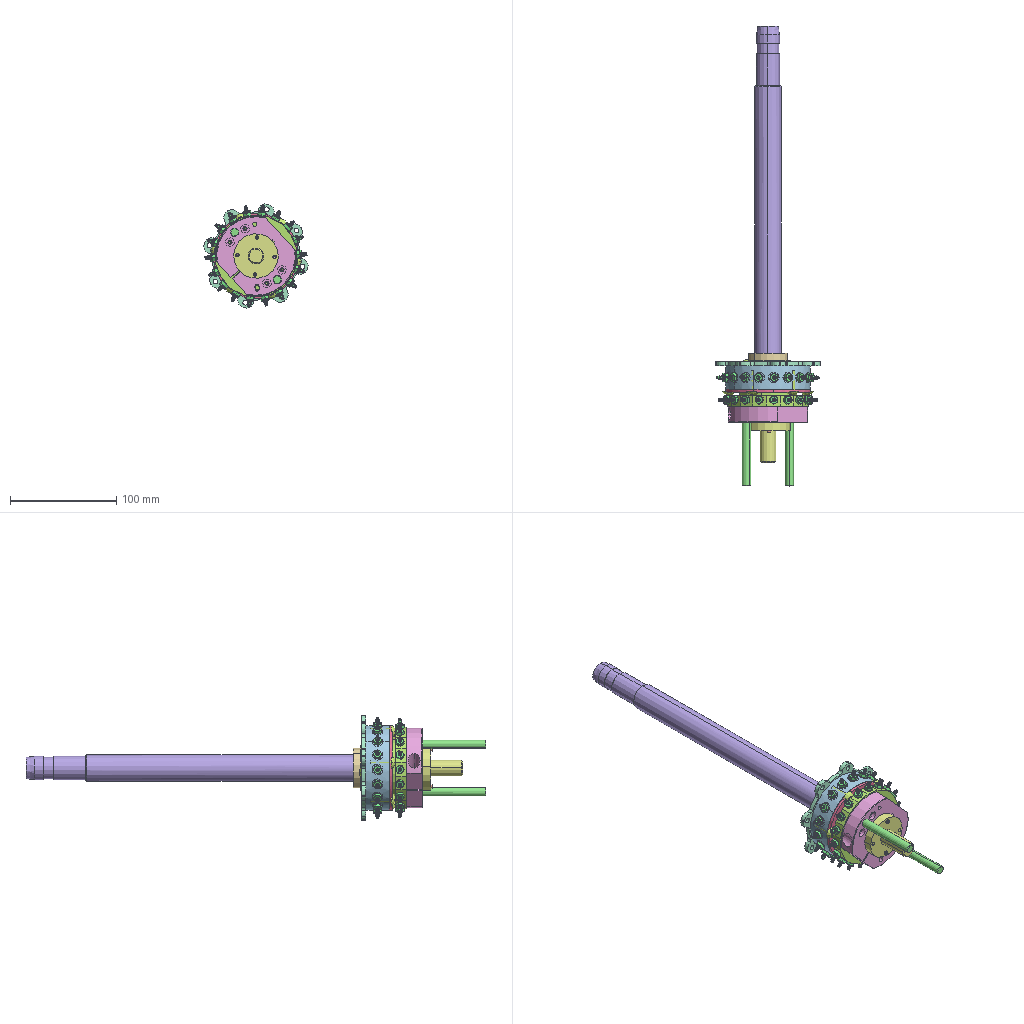Assembly | SolidWorks | 25 different items | 116 placed | box 98 x 433 x 98 mm
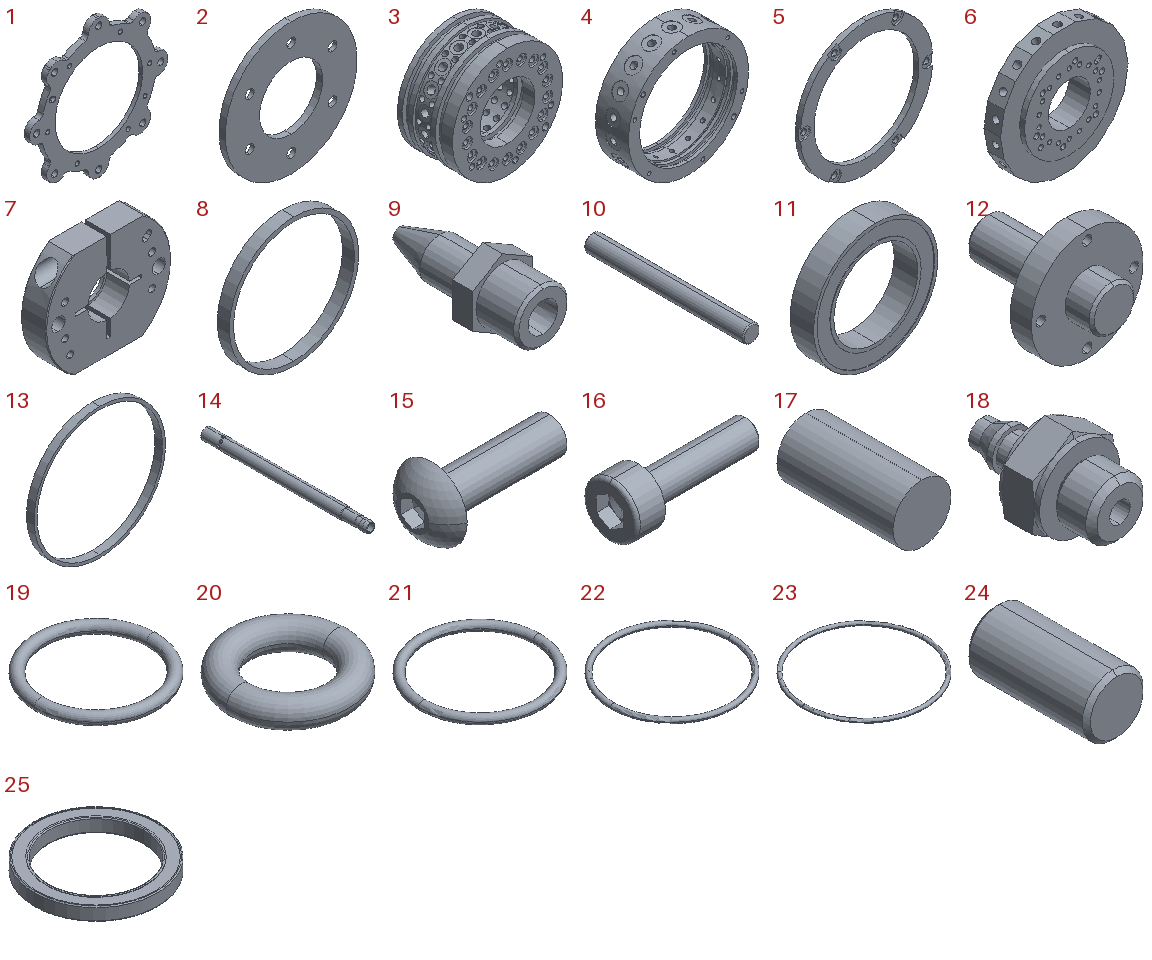Parts list (item | quantity | size | volume | features):
1 | x1 | 100 x 4 x 100 mm | 10292 mm3 | features ICE 11, CirPattern 3, Fillet 2, Extrusion 1
2 | x1 | 52.5 x 2.5 x 52.5 mm | 3777 mm3 | features ICE 4, CirPattern 2, Chamfer 1, Extrusion 1
3 | x1 | 50 x 25 x 50 mm | 28729 mm3 | features ICE 10, CirPattern 7, RevCut 4, 3DProfileFeature 3, HoleWzd 3, Extrusion 1
4 | x1 | 80 x 22 x 80 mm | 34396 mm3 | features ICE 6, CirPattern 5, 3DProfileFeature 3, HoleWzd 3, RevCut 2, Cut 1, Extrusion 1, Revolution 1
5 | x1 | 80 x 3 x 80 mm | 5249 mm3 | features CirPattern 3, ICE 2, Cut 1, Extrusion 1
6 | x1 | 77.172 x 13 x 76 mm | 40512 mm3 | features ICE 12, CirPattern 5, HoleWzd 2, 3DProfileFeature 1, Chamfer 1, Cut 1, Extrusion 1
7 | x1 | 75 x 15 x 62 mm | 46080 mm3 | features ICE 12, 3DProfileFeature 2, HoleWzd 2, Chamfer 1, CirPattern 1, Extrusion 1
8 | x1 | 27 x 2.5 x 27 mm | 184.49 mm3 | features Extrusion 1
9 | x18 | 4.5 x 10.7 x 5.196 mm | 80.12 mm3 | features ICE 4, Chamfer 2, Extrusion 1, RevCut 1
10 | x2 | 8 x 75 x 8 mm | 3753 mm3 | features Chamfer 1, Extrusion 1, ICE 1
11 | x1 | 37 x 7 x 37 mm | 3935 mm3 | features ICE 2, Extrusion 1
12 | x1 | 42 x 48 x 42 mm | 18246 mm3 | features ICE 10, Chamfer 2, CirPattern 2, Extrusion 1
13 | x1 | 52.5 x 3 x 52.5 mm | 556.557 mm3 | features Extrusion 1
14 | x1 | 25 x 371 x 25 mm | 90004 mm3 | features Chamfer 3, ICE 3, CirPattern 2, Extrusion 1, RefAxis 1, RevCut 1
15 | x14 | 23.3 x 12 x 12 mm | 775.96 mm3 | features Cut 2, RevCut 2, Boss 1, Extrusion 1, Fillet 1, LPattern 1
16 | x2 | 7.6 x 3 x 3 mm | 21.652 mm3 | features Fillet 2, RevCut 2, Boss 1, Chamfer 1, Cut 1, Extrusion 1, LPattern 1
17 | x2 | 4 x 8 x 4 mm | 100.531 mm3 | features Extrusion 1
18 | x36 | 7 x 12 x 8.083 mm | 212.301 mm3 | features BaseBody 1
19 | x1 | 22 x 22 x 2 mm | 197.392 mm3 | features RefAxis 1, Revolution 1
20 | x18 | 4.6 x 4.6 x 1 mm | 8.883 mm3 | features RefAxis 1, Revolution 1
21 | x2 | 29 x 29 x 2 mm | 266.479 mm3 | features RefAxis 1, Revolution 1
22 | x2 | 50 x 50 x 2 mm | 473.741 mm3 | features RefAxis 1, Revolution 1
23 | x2 | 69 x 69 x 2 mm | 661.263 mm3 | features RefAxis 1, Revolution 1
24 | x3 | 3 x 6 x 3 mm | 42.051 mm3 | features Chamfer 1, Extrusion 1
25 | x2 | 65 x 65 x 7 mm | 9064 mm3 | features Extrusion 1, Fillet 1, ICE 1, MirrorPattern 1
Mates (type | each side: item.copy, entity, surface, feature):
DistanceDim | 3.1 face plane Boss-Extrude1 | 2.1 face plane Boss-Extrude1
Concentric | 2.1 face cylinder Boss-Extrude1 | 3.1 face cylinder Boss-Extrude1
Concentric | 2.1 face cylinder CirPattern1 | 3.1 face cylinder M3 Tapped Hole1
Coincident | 2.1 face plane Boss-Extrude1 | 25.1 face plane Boss-Extrude1
Coincident | 4.1 face plane Boss-Extrude1 | 5.1 face plane Boss-Extrude1
Concentric | 4.1 face cylinder Boss-Extrude1 | 5.1 face cylinder Boss-Extrude1
Concentric | 4.1 face cylinder Boss-Extrude1 | 25.2 face cylinder Boss-Extrude1
Coincident | 4.1 face plane Revolve1 | 25.2 face plane Boss-Extrude1
Coincident | 4.1 face plane Revolve1 | 25.1 face plane Boss-Extrude1
Concentric | 4.1 face cylinder Boss-Extrude1 | 25.1 face cylinder Boss-Extrude1
Concentric | 3.1 face cylinder Boss-Extrude1 | 25.2 face cylinder Boss-Extrude1
Concentric | 7.1 face cylinder Cut-Extrude8 | 10.1 face cylinder Boss-Extrude1
Coincident | 10.1 face plane Boss-Extrude1 | 10.2 face plane Boss-Extrude1
DistanceDim | 10.2 face plane Boss-Extrude1 | 6.1 face plane Boss-Extrude3
Coincident | 4.1 face plane CirPattern2 | 18.1 face plane Input 1
Concentric | 4.1 face cylinder CirPattern3 | 18.1 face cylinder Input 1
Coincident | 6.1 face plane Boss-Extrude3 | 18.2 face plane Input 1
Concentric | 6.1 face cylinder CirPattern14 | 18.2 face cylinder Input 1
Coincident | 12.1 face plane Boss-Extrude1 | 16.1 face plane BaseHead
Coincident | 12.1 face plane Boss-Extrude1 | 16.2 face plane BaseHead
Coincident | 3.1 face plane CirPattern6 | 9.1 face plane Boss-Extrude2
DistanceDim | 22.1 plane | 3.1 face plane Cut-Revolve2
DistanceDim | 22.2 plane | 3.1 face plane Cut-Revolve2
DistanceDim | 23.1 plane | 4.1 face plane Cut-Revolve3
DistanceDim | 23.2 plane | 4.1 face plane Cut-Revolve3
Concentric | 3.1 face cylinder CirPattern11 | 9.1 face cylinder Boss-Extrude3
DistanceDim | 3.1 face plane CirPattern13 | 20.1 plane
Concentric | 3.1 edge | 20.1 axis
Coincident | 3.1 face plane Cut-Extrude12 | 24.1 face plane Boss-Extrude1
Concentric | 3.1 face cylinder Cut-Extrude12 | 24.1 face cylinder Boss-Extrude1
Coincident | 3.1 face plane Cut-Extrude12 | 24.2 face plane Boss-Extrude1
Concentric | 3.1 face cylinder Cut-Extrude12 | 24.2 face cylinder Boss-Extrude1
Parallel | 4.1 face plane CirPattern2 | 6.1 face plane Boss-Extrude3
Coincident | 4.1 face plane Cut-Extrude7 | 24.3 face plane Boss-Extrude1
Concentric | 4.1 face cylinder Cut-Extrude7 | 24.3 face cylinder Boss-Extrude1
Coincident | 1.1 face plane Boss-Extrude1 | 4.1 face plane Boss-Extrude1
Concentric | 1.1 face cylinder Cut-Extrude1 | 4.1 face cylinder Boss-Extrude1
Coincident | 6.1 face plane Cut-Extrude14 | 17.1 face plane Boss-Extrude1
Concentric | 6.1 face cylinder Cut-Extrude14 | 17.1 face cylinder Boss-Extrude1
Coincident | 6.1 face plane Cut-Extrude14 | 17.2 face plane Boss-Extrude1
Concentric | 6.1 face cylinder Cut-Extrude14 | 17.2 face cylinder Boss-Extrude1
Concentric | 3.1 edge | 21.1 axis
DistanceDim | 21.1 plane | 3.1 face plane Cut-Revolve3
Concentric | 3.1 edge | 21.2 axis
DistanceDim | 21.2 plane | 3.1 face plane Cut-Revolve3
Concentric | 3.1 face cylinder Boss-Extrude1 | 13.1 face cylinder Boss-Extrude1
Concentric | 2.1 face cylinder Cut-Extrude2 | 15.1 face cylinder BaseBody
Coincident | 2.1 face plane Cut-Extrude3 | 15.1 face plane BaseHead
Concentric | 2.1 face cylinder CirPattern1 | 15.2 face cylinder BaseBody
Coincident | 2.1 face plane CirPattern2 | 15.2 face plane BaseHead
Concentric | 2.1 face cylinder CirPattern1 | 15.3 face cylinder BaseBody
Coincident | 2.1 face plane CirPattern2 | 15.3 face plane BaseHead
Concentric | 2.1 face cylinder CirPattern1 | 15.4 face cylinder BaseBody
Coincident | 2.1 face plane CirPattern2 | 15.4 face plane BaseHead
Concentric | 2.1 face cylinder CirPattern1 | 15.5 face cylinder BaseBody
Coincident | 2.1 face plane CirPattern2 | 15.5 face plane BaseHead
Concentric | 2.1 face cylinder CirPattern2 | 15.6 face cylinder BaseBody
Coincident | 2.1 face plane Cut-Extrude1 | 15.6 face plane BaseHead
Concentric | 3.1 face cylinder Cut-Extrude1 | 6.1 face cylinder Boss-Extrude1
Concentric | 3.1 face cylinder Cut-Extrude12 | 6.1 face cylinder Cut-Extrude12
Coincident | 3.1 face plane Boss-Extrude2 | 6.1 face plane Cut-Extrude13
Concentric | 3.1 face cylinder Cut-Revolve4 | 14.1 face cylinder Boss-Extrude1
DistanceDim | 19.1 plane | 14.1 face plane Boss-Extrude1
Concentric | 6.1 face cylinder Cut-Extrude9 | 15.7 face cylinder BaseBody
Concentric | 6.1 face cylinder Cut-Extrude9 | 15.8 face cylinder BaseBody
Coincident | 6.1 face plane Cut-Extrude9 | 15.7 face plane BaseHead
Coincident | 6.1 face plane Cut-Extrude9 | 15.8 face plane BaseHead
Concentric | 5.1 face cylinder Cut-Extrude2 | 15.9 face cylinder BaseBody
Coincident | 5.1 face plane CirPattern2 | 15.9 face plane BaseHead
Concentric | 5.1 face cylinder CirPattern1 | 15.10 face cylinder BaseBody
Coincident | 5.1 face plane CirPattern2 | 15.10 face plane BaseHead
Concentric | 5.1 face cylinder CirPattern1 | 15.11 face cylinder BaseBody
Coincident | 5.1 face plane CirPattern2 | 15.11 face plane BaseHead
Concentric | 5.1 face cylinder CirPattern1 | 15.12 face cylinder BaseBody
Coincident | 5.1 face plane CirPattern2 | 15.12 face plane BaseHead
Concentric | 5.1 face cylinder CirPattern1 | 15.13 face cylinder BaseBody
Coincident | 5.1 face plane CirPattern2 | 15.13 face plane BaseHead
Concentric | 5.1 face cylinder CirPattern1 | 15.14 face cylinder BaseBody
Coincident | 5.1 face plane Cut-Extrude4 | 15.14 face plane BaseHead
Concentric | 12.1 face cylinder Boss-Extrude6 | 8.1 edge
Coincident | 11.1 face plane Boss-Extrude1 | 8.1 face plane Boss-Extrude1
Concentric | 7.1 face cylinder Boss-Extrude1 | 14.1 face cylinder Boss-Extrude1
Coincident | 6.1 face plane Boss-Extrude3 | 7.1 face plane Boss-Extrude1
PlanarAngleDim | 7.1 plane | assembly plane
Concentric | 7.1 face cylinder Cut-Extrude8 | 10.2 face cylinder Boss-Extrude1
Coincident | 7.1 face plane Boss-Extrude1 | 12.1 face plane Boss-Extrude7
Concentric | 4.1 face cylinder CirPattern4 | 1.1 face cylinder Cut-Extrude5